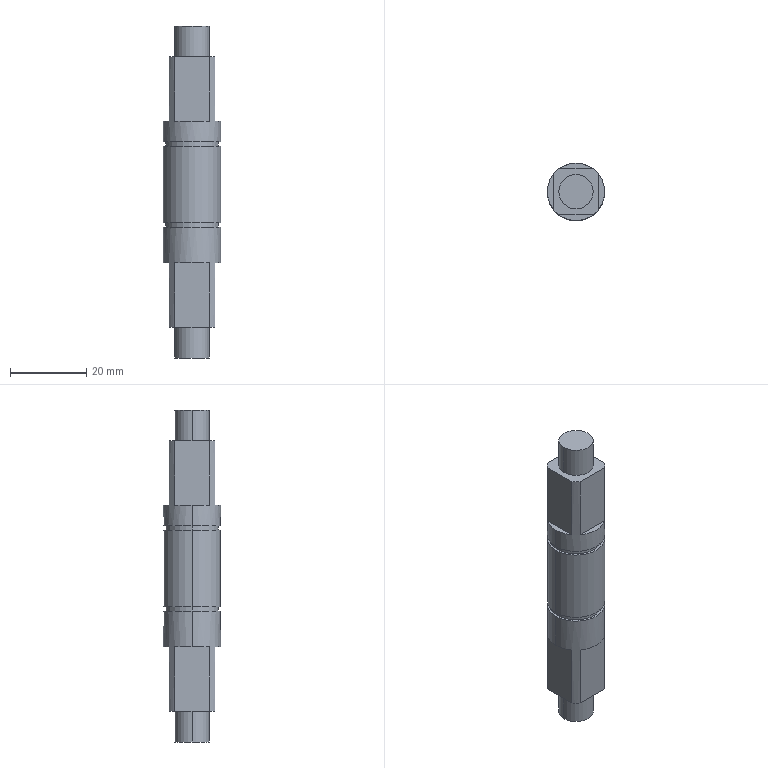Part | STEP file | Connecting shaft QY-1-03 | 1 solid | 38 faces | box 15 x 15 x 87 mm | volume 12249 mm3 | plane 24 | cylinder 14 | commonest cylinder face diameters 15 x6 9 x4 13.8 x4